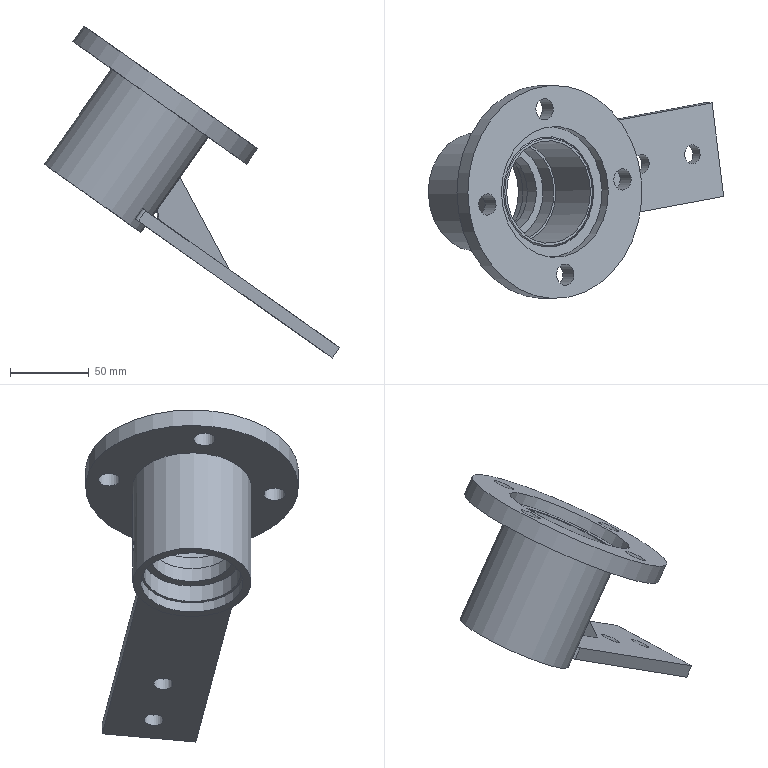Part | STEP file | HL4GZ-1.862.046 (motor mounting seat) | 4 solids | 42 faces | box 187.193 x 135 x 210.336 mm | volume 284411 mm3 | plane 21 | cylinder 20 | cone 1 | commonest cylinder face diameters 13.5 x4 4 x2 12 x2 62 x2 65 x2 70 x2